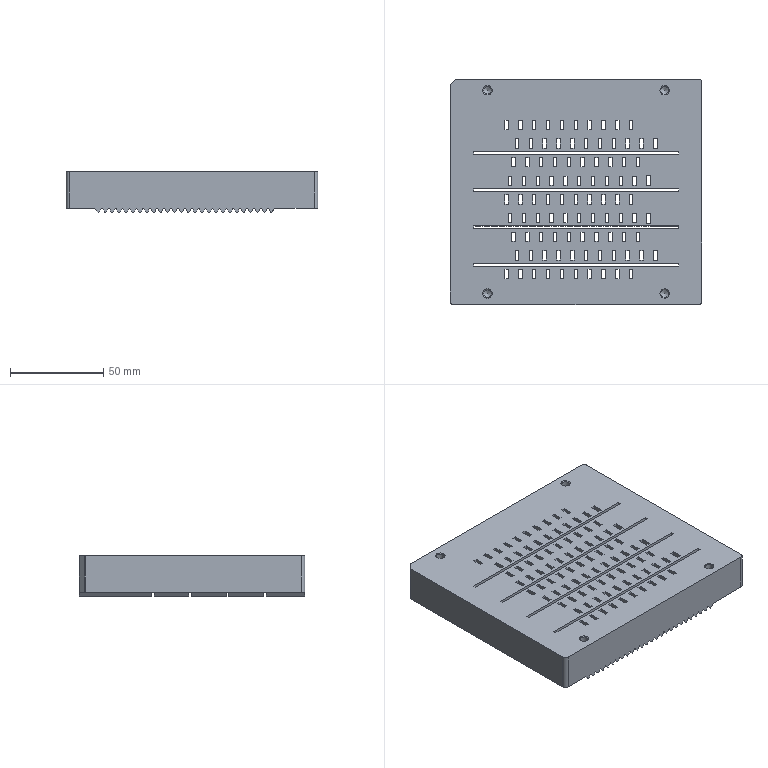Part | STEP file | 200 mesh_id2074 | 1 solid | 1028 faces | box 135 x 121 x 21.89 mm | volume 302642 mm3 | plane 660 | cylinder 358 | cone 8 | torus 2 | commonest cylinder face diameters 0.5 x349 4.2 x4 4 x3 1 x2